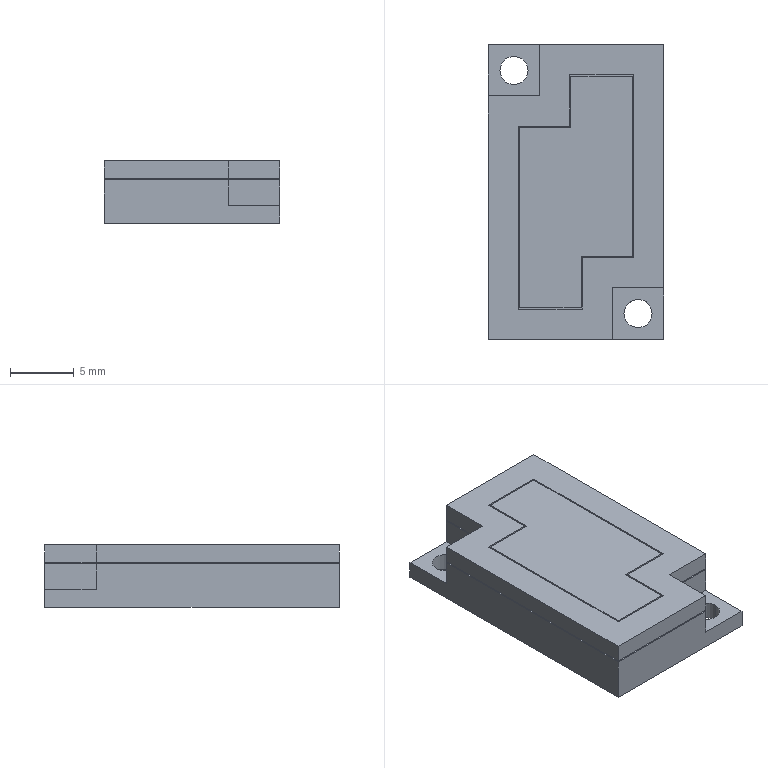Part | SolidWorks | features HoleWzd 2, BaseBody 1, ICE 1 | 1 solid | 52 faces | box 13.7 x 23 x 4.9 mm | volume 1409 mm3 | plane 48 | cylinder 4 | commonest cylinder face diameters 2.2 x4
STEP:
#1=CARTESIAN_POINT('',(8.6,-19.,0.));
#2=VERTEX_POINT('',#1);
#3=CARTESIAN_POINT('',(10.8,-19.,0.));
#4=VERTEX_POINT('',#3);
#5=CARTESIAN_POINT('',(9.7,-19.,0.));
#6=DIRECTION('',(0.,0.,1.));
#7=DIRECTION('',(1.,0.,0.));
#8=AXIS2_PLACEMENT_3D('',#5,#6,#7);
#9=CIRCLE('',#8,1.1);
#10=EDGE_CURVE('',#2,#4,#9,.T.);
#11=ORIENTED_EDGE('',*,*,#10,.F.);
#12=CARTESIAN_POINT('',(8.6,-19.,1.4));
#13=VERTEX_POINT('',#12);
#14=CARTESIAN_POINT('',(8.6,-19.,1.4));
#15=DIRECTION('',(0.,0.,1.));
#16=VECTOR('',#15,1000.);
#17=LINE('',#14,#16);
#18=EDGE_CURVE('',#2,#13,#17,.T.);
#19=ORIENTED_EDGE('',*,*,#18,.T.);
#20=CARTESIAN_POINT('',(10.8,-19.,1.4));
#21=VERTEX_POINT('',#20);
#22=CARTESIAN_POINT('',(9.7,-19.,1.4));
#23=DIRECTION('',(0.,0.,1.));
#24=DIRECTION('',(1.,0.,0.));
#25=AXIS2_PLACEMENT_3D('',#22,#23,#24);
#26=CIRCLE('',#25,1.1);
#27=EDGE_CURVE('',#13,#21,#26,.T.);
#28=ORIENTED_EDGE('',*,*,#27,.T.);
#29=CARTESIAN_POINT('',(10.8,-19.,1.4));
#30=DIRECTION('',(0.,0.,1.));
#31=VECTOR('',#30,1000.);
#32=LINE('',#29,#31);
#33=EDGE_CURVE('',#4,#21,#32,.T.);
#34=ORIENTED_EDGE('',*,*,#33,.F.);
#35=EDGE_LOOP('',(#11,#19,#28,#34));
#36=FACE_OUTER_BOUND('',#35,.T.);
#37=CARTESIAN_POINT('',(9.7,-19.,1.4));
#38=DIRECTION('',(0.,0.,1.));
#39=DIRECTION('',(1.,0.,0.));
#40=AXIS2_PLACEMENT_3D('',#37,#38,#39);
#41=CYLINDRICAL_SURFACE('',#40,1.1);
#42=ADVANCED_FACE('',(#36),#41,.F.);
#43=CARTESIAN_POINT('',(-1.1,0.,0.));
#44=VERTEX_POINT('',#43);
#45=CARTESIAN_POINT('',(1.1,0.,0.));
#46=VERTEX_POINT('',#45);
#47=CARTESIAN_POINT('',(0.,0.,0.));
#48=DIRECTION('',(0.,0.,1.));
#49=DIRECTION('',(1.,0.,0.));
#50=AXIS2_PLACEMENT_3D('',#47,#48,#49);
#51=CIRCLE('',#50,1.1);
#52=EDGE_CURVE('',#44,#46,#51,.T.);
#53=ORIENTED_EDGE('',*,*,#52,.F.);
#54=CARTESIAN_POINT('',(-1.1,0.,1.4));
#55=VERTEX_POINT('',#54);
#56=CARTESIAN_POINT('',(-1.1,0.,1.4));
#57=DIRECTION('',(0.,0.,1.));
#58=VECTOR('',#57,1000.);
#59=LINE('',#56,#58);
#60=EDGE_CURVE('',#44,#55,#59,.T.);
#61=ORIENTED_EDGE('',*,*,#60,.T.);
#62=CARTESIAN_POINT('',(1.1,0.,1.4));
#63=VERTEX_POINT('',#62);
#64=CARTESIAN_POINT('',(0.,0.,1.4));
#65=DIRECTION('',(0.,0.,1.));
#66=DIRECTION('',(1.,0.,0.));
#67=AXIS2_PLACEMENT_3D('',#64,#65,#66);
#68=CIRCLE('',#67,1.1);
#69=EDGE_CURVE('',#55,#63,#68,.T.);
#70=ORIENTED_EDGE('',*,*,#69,.T.);
#71=CARTESIAN_POINT('',(1.1,0.,1.4));
#72=DIRECTION('',(0.,0.,1.));
#73=VECTOR('',#72,1000.);
#74=LINE('',#71,#73);
#75=EDGE_CURVE('',#46,#63,#74,.T.);
#76=ORIENTED_EDGE('',*,*,#75,.F.);
#77=EDGE_LOOP('',(#53,#61,#70,#76));
#78=FACE_OUTER_BOUND('',#77,.T.);
#79=CARTESIAN_POINT('',(0.,0.,1.4));
#80=DIRECTION('',(0.,0.,1.));
#81=DIRECTION('',(1.,0.,0.));
#82=AXIS2_PLACEMENT_3D('',#79,#80,#81);
#83=CYLINDRICAL_SURFACE('',#82,1.1);
#84=ADVANCED_FACE('',(#78),#83,.F.);
#85=CARTESIAN_POINT('',(-2.,-2.,3.5));
#86=VERTEX_POINT('',#85);
#87=CARTESIAN_POINT('',(-2.,-21.,3.5));
#88=VERTEX_POINT('',#87);
#89=CARTESIAN_POINT('',(-2.,-2.,3.5));
#90=DIRECTION('',(0.,-1.,0.));
#91=VECTOR('',#90,1000.);
#92=LINE('',#89,#91);
#93=EDGE_CURVE('',#86,#88,#92,.T.);
#94=ORIENTED_EDGE('',*,*,#93,.T.);
#95=CARTESIAN_POINT('',(-2.,-21.,4.9));
#96=VERTEX_POINT('',#95);
#97=CARTESIAN_POINT('',(-2.,-21.,1.4));
#98=DIRECTION('',(0.,0.,-1.));
#99=VECTOR('',#98,1000.);
#100=LINE('',#97,#99);
#101=EDGE_CURVE('',#96,#88,#100,.T.);
#102=ORIENTED_EDGE('',*,*,#101,.F.);
#103=CARTESIAN_POINT('',(-2.,-2.,4.9));
#104=VERTEX_POINT('',#103);
#105=CARTESIAN_POINT('',(-2.,-2.,4.9));
#106=DIRECTION('',(0.,-1.,0.));
#107=VECTOR('',#106,1000.);
#108=LINE('',#105,#107);
#109=EDGE_CURVE('',#104,#96,#108,.T.);
#110=ORIENTED_EDGE('',*,*,#109,.F.);
#111=CARTESIAN_POINT('',(-2.,-2.,4.9));
#112=DIRECTION('',(0.,0.,-1.));
#113=VECTOR('',#112,1000.);
#114=LINE('',#111,#113);
#115=EDGE_CURVE('',#104,#86,#114,.T.);
#116=ORIENTED_EDGE('',*,*,#115,.T.);
#117=EDGE_LOOP('',(#94,#102,#110,#116));
#118=FACE_OUTER_BOUND('',#117,.T.);
#119=CARTESIAN_POINT('',(-2.,2.,1.4));
#120=DIRECTION('',(1.,0.,0.));
#121=DIRECTION('',(0.,1.,0.));
#122=AXIS2_PLACEMENT_3D('',#119,#120,#121);
#123=PLANE('',#122);
#124=ADVANCED_FACE('',(#118),#123,.F.);
#125=CARTESIAN_POINT('',(7.7,-21.,3.5));
#126=VERTEX_POINT('',#125);
#127=CARTESIAN_POINT('',(-2.,-21.,3.5));
#128=DIRECTION('',(1.,0.,0.));
#129=VECTOR('',#128,1000.);
#130=LINE('',#127,#129);
#131=EDGE_CURVE('',#88,#126,#130,.T.);
#132=ORIENTED_EDGE('',*,*,#131,.T.);
#133=CARTESIAN_POINT('',(7.7,-21.,4.9));
#134=VERTEX_POINT('',#133);
#135=CARTESIAN_POINT('',(7.7,-21.,4.9));
#136=DIRECTION('',(0.,0.,-1.));
#137=VECTOR('',#136,1000.);
#138=LINE('',#135,#137);
#139=EDGE_CURVE('',#134,#126,#138,.T.);
#140=ORIENTED_EDGE('',*,*,#139,.F.);
#141=CARTESIAN_POINT('',(-2.,-21.,4.9));
#142=DIRECTION('',(1.,0.,0.));
#143=VECTOR('',#142,1000.);
#144=LINE('',#141,#143);
#145=EDGE_CURVE('',#96,#134,#144,.T.);
#146=ORIENTED_EDGE('',*,*,#145,.F.);
#147=ORIENTED_EDGE('',*,*,#101,.T.);
#148=EDGE_LOOP('',(#132,#140,#146,#147));
#149=FACE_OUTER_BOUND('',#148,.T.);
#150=CARTESIAN_POINT('',(-2.,-21.,1.4));
#151=DIRECTION('',(0.,1.,0.));
#152=DIRECTION('',(-1.,0.,0.));
#153=AXIS2_PLACEMENT_3D('',#150,#151,#152);
#154=PLANE('',#153);
#155=ADVANCED_FACE('',(#149),#154,.F.);
#156=CARTESIAN_POINT('',(11.7,-17.,3.5));
#157=VERTEX_POINT('',#156);
#158=CARTESIAN_POINT('',(11.7,2.,3.5));
#159=VERTEX_POINT('',#158);
#160=CARTESIAN_POINT('',(11.7,-17.,3.5));
#161=DIRECTION('',(0.,1.,0.));
#162=VECTOR('',#161,1000.);
#163=LINE('',#160,#162);
#164=EDGE_CURVE('',#157,#159,#163,.T.);
#165=ORIENTED_EDGE('',*,*,#164,.T.);
#166=CARTESIAN_POINT('',(11.7,2.,4.9));
#167=VERTEX_POINT('',#166);
#168=CARTESIAN_POINT('',(11.7,2.,1.4));
#169=DIRECTION('',(0.,0.,-1.));
#170=VECTOR('',#169,1000.);
#171=LINE('',#168,#170);
#172=EDGE_CURVE('',#167,#159,#171,.T.);
#173=ORIENTED_EDGE('',*,*,#172,.F.);
#174=CARTESIAN_POINT('',(11.7,-17.,4.9));
#175=VERTEX_POINT('',#174);
#176=CARTESIAN_POINT('',(11.7,-17.,4.9));
#177=DIRECTION('',(0.,1.,0.));
#178=VECTOR('',#177,1000.);
#179=LINE('',#176,#178);
#180=EDGE_CURVE('',#175,#167,#179,.T.);
#181=ORIENTED_EDGE('',*,*,#180,.F.);
#182=CARTESIAN_POINT('',(11.7,-17.,4.9));
#183=DIRECTION('',(0.,0.,-1.));
#184=VECTOR('',#183,1000.);
#185=LINE('',#182,#184);
#186=EDGE_CURVE('',#175,#157,#185,.T.);
#187=ORIENTED_EDGE('',*,*,#186,.T.);
#188=EDGE_LOOP('',(#165,#173,#181,#187));
#189=FACE_OUTER_BOUND('',#188,.T.);
#190=CARTESIAN_POINT('',(11.7,2.,1.4));
#191=DIRECTION('',(-1.,0.,0.));
#192=DIRECTION('',(0.,-1.,0.));
#193=AXIS2_PLACEMENT_3D('',#190,#191,#192);
#194=PLANE('',#193);
#195=ADVANCED_FACE('',(#189),#194,.F.);
#196=CARTESIAN_POINT('',(2.,2.,3.5));
#197=VERTEX_POINT('',#196);
#198=CARTESIAN_POINT('',(11.7,2.,3.5));
#199=DIRECTION('',(-1.,0.,0.));
#200=VECTOR('',#199,1000.);
#201=LINE('',#198,#200);
#202=EDGE_CURVE('',#159,#197,#201,.T.);
#203=ORIENTED_EDGE('',*,*,#202,.T.);
#204=CARTESIAN_POINT('',(2.,2.,4.9));
#205=VERTEX_POINT('',#204);
#206=CARTESIAN_POINT('',(2.,2.,4.9));
#207=DIRECTION('',(0.,0.,-1.));
#208=VECTOR('',#207,1000.);
#209=LINE('',#206,#208);
#210=EDGE_CURVE('',#205,#197,#209,.T.);
#211=ORIENTED_EDGE('',*,*,#210,.F.);
#212=CARTESIAN_POINT('',(11.7,2.,4.9));
#213=DIRECTION('',(-1.,0.,0.));
#214=VECTOR('',#213,1000.);
#215=LINE('',#212,#214);
#216=EDGE_CURVE('',#167,#205,#215,.T.);
#217=ORIENTED_EDGE('',*,*,#216,.F.);
#218=ORIENTED_EDGE('',*,*,#172,.T.);
#219=EDGE_LOOP('',(#203,#211,#217,#218));
#220=FACE_OUTER_BOUND('',#219,.T.);
#221=CARTESIAN_POINT('',(-2.,2.,1.4));
#222=DIRECTION('',(0.,-1.,0.));
#223=DIRECTION('',(1.,0.,0.));
#224=AXIS2_PLACEMENT_3D('',#221,#222,#223);
#225=PLANE('',#224);
#226=ADVANCED_FACE('',(#220),#225,.F.);
#227=CARTESIAN_POINT('',(7.7,-17.,3.5));
#228=VERTEX_POINT('',#227);
#229=CARTESIAN_POINT('',(7.7,-21.,3.5));
#230=DIRECTION('',(0.,1.,0.));
#231=VECTOR('',#230,1000.);
#232=LINE('',#229,#231);
#233=EDGE_CURVE('',#126,#228,#232,.T.);
#234=ORIENTED_EDGE('',*,*,#233,.T.);
#235=CARTESIAN_POINT('',(7.7,-17.,4.9));
#236=VERTEX_POINT('',#235);
#237=CARTESIAN_POINT('',(7.7,-17.,4.9));
#238=DIRECTION('',(0.,0.,-1.));
#239=VECTOR('',#238,1000.);
#240=LINE('',#237,#239);
#241=EDGE_CURVE('',#236,#228,#240,.T.);
#242=ORIENTED_EDGE('',*,*,#241,.F.);
#243=CARTESIAN_POINT('',(7.7,-17.,4.9));
#244=DIRECTION('',(0.,1.,0.));
#245=VECTOR('',#244,1000.);
#246=LINE('',#243,#245);
#247=EDGE_CURVE('',#134,#236,#246,.T.);
#248=ORIENTED_EDGE('',*,*,#247,.F.);
#249=ORIENTED_EDGE('',*,*,#139,.T.);
#250=EDGE_LOOP('',(#234,#242,#248,#249));
#251=FACE_OUTER_BOUND('',#250,.T.);
#252=CARTESIAN_POINT('',(7.7,-17.,4.9));
#253=DIRECTION('',(-1.,0.,0.));
#254=DIRECTION('',(0.,0.,1.));
#255=AXIS2_PLACEMENT_3D('',#252,#253,#254);
#256=PLANE('',#255);
#257=ADVANCED_FACE('',(#251),#256,.F.);
#258=CARTESIAN_POINT('',(7.7,-17.,3.5));
#259=DIRECTION('',(1.,0.,0.));
#260=VECTOR('',#259,1000.);
#261=LINE('',#258,#260);
#262=EDGE_CURVE('',#228,#157,#261,.T.);
#263=ORIENTED_EDGE('',*,*,#262,.T.);
#264=ORIENTED_EDGE('',*,*,#186,.F.);
#265=CARTESIAN_POINT('',(7.7,-17.,4.9));
#266=DIRECTION('',(1.,0.,0.));
#267=VECTOR('',#266,1000.);
#268=LINE('',#265,#267);
#269=EDGE_CURVE('',#236,#175,#268,.T.);
#270=ORIENTED_EDGE('',*,*,#269,.F.);
#271=ORIENTED_EDGE('',*,*,#241,.T.);
#272=EDGE_LOOP('',(#263,#264,#270,#271));
#273=FACE_OUTER_BOUND('',#272,.T.);
#274=CARTESIAN_POINT('',(7.7,-17.,4.9));
#275=DIRECTION('',(0.,1.,0.));
#276=DIRECTION('',(0.,0.,1.));
#277=AXIS2_PLACEMENT_3D('',#274,#275,#276);
#278=PLANE('',#277);
#279=ADVANCED_FACE('',(#273),#278,.F.);
#280=CARTESIAN_POINT('',(2.,-2.,3.5));
#281=VERTEX_POINT('',#280);
#282=CARTESIAN_POINT('',(2.,2.,3.5));
#283=DIRECTION('',(0.,-1.,0.));
#284=VECTOR('',#283,1000.);
#285=LINE('',#282,#284);
#286=EDGE_CURVE('',#197,#281,#285,.T.);
#287=ORIENTED_EDGE('',*,*,#286,.T.);
#288=CARTESIAN_POINT('',(2.,-2.,4.9));
#289=VERTEX_POINT('',#288);
#290=CARTESIAN_POINT('',(2.,-2.,4.9));
#291=DIRECTION('',(0.,0.,-1.));
#292=VECTOR('',#291,1000.);
#293=LINE('',#290,#292);
#294=EDGE_CURVE('',#289,#281,#293,.T.);
#295=ORIENTED_EDGE('',*,*,#294,.F.);
#296=CARTESIAN_POINT('',(2.,2.,4.9));
#297=DIRECTION('',(0.,-1.,0.));
#298=VECTOR('',#297,1000.);
#299=LINE('',#296,#298);
#300=EDGE_CURVE('',#205,#289,#299,.T.);
#301=ORIENTED_EDGE('',*,*,#300,.F.);
#302=ORIENTED_EDGE('',*,*,#210,.T.);
#303=EDGE_LOOP('',(#287,#295,#301,#302));
#304=FACE_OUTER_BOUND('',#303,.T.);
#305=CARTESIAN_POINT('',(2.,2.,4.9));
#306=DIRECTION('',(1.,0.,0.));
#307=DIRECTION('',(0.,1.,0.));
#308=AXIS2_PLACEMENT_3D('',#305,#306,#307);
#309=PLANE('',#308);
#310=ADVANCED_FACE('',(#304),#309,.F.);
#311=CARTESIAN_POINT('',(2.,-2.,3.5));
#312=DIRECTION('',(-1.,0.,0.));
#313=VECTOR('',#312,1000.);
#314=LINE('',#311,#313);
#315=EDGE_CURVE('',#281,#86,#314,.T.);
#316=ORIENTED_EDGE('',*,*,#315,.T.);
#317=ORIENTED_EDGE('',*,*,#115,.F.);
#318=CARTESIAN_POINT('',(2.,-2.,4.9));
#319=DIRECTION('',(-1.,0.,0.));
#320=VECTOR('',#319,1000.);
#321=LINE('',#318,#320);
#322=EDGE_CURVE('',#289,#104,#321,.T.);
#323=ORIENTED_EDGE('',*,*,#322,.F.);
#324=ORIENTED_EDGE('',*,*,#294,.T.);
#325=EDGE_LOOP('',(#316,#317,#323,#324));
#326=FACE_OUTER_BOUND('',#325,.T.);
#327=CARTESIAN_POINT('',(2.,-2.,4.9));
#328=DIRECTION('',(0.,-1.,0.));
#329=DIRECTION('',(1.,0.,0.));
#330=AXIS2_PLACEMENT_3D('',#327,#328,#329);
#331=PLANE('',#330);
#332=ADVANCED_FACE('',(#326),#331,.F.);
#333=CARTESIAN_POINT('',(0.35,-4.35,4.9));
#334=VERTEX_POINT('',#333);
#335=CARTESIAN_POINT('',(0.35,-18.65,4.9));
#336=VERTEX_POINT('',#335);
#337=CARTESIAN_POINT('',(0.35,-4.45,4.9));
#338=DIRECTION('',(0.,-1.,0.));
#339=VECTOR('',#338,1000.);
#340=LINE('',#337,#339);
#341=EDGE_CURVE('',#334,#336,#340,.T.);
#342=ORIENTED_EDGE('',*,*,#341,.F.);
#343=CARTESIAN_POINT('',(4.35,-4.35,4.9));
#344=VERTEX_POINT('',#343);
#345=CARTESIAN_POINT('',(0.45,-4.35,4.9));
#346=DIRECTION('',(-1.,0.,0.));
#347=VECTOR('',#346,1000.);
#348=LINE('',#345,#347);
#349=EDGE_CURVE('',#344,#334,#348,.T.);
#350=ORIENTED_EDGE('',*,*,#349,.F.);
#351=CARTESIAN_POINT('',(4.35,-0.35,4.9));
#352=VERTEX_POINT('',#351);
#353=CARTESIAN_POINT('',(4.35,-4.45,4.9));
#354=DIRECTION('',(0.,-1.,0.));
#355=VECTOR('',#354,1000.);
#356=LINE('',#353,#355);
#357=EDGE_CURVE('',#352,#344,#356,.T.);
#358=ORIENTED_EDGE('',*,*,#357,.F.);
#359=CARTESIAN_POINT('',(9.35,-0.35,4.9));
#360=VERTEX_POINT('',#359);
#361=CARTESIAN_POINT('',(0.45,-0.35,4.9));
#362=DIRECTION('',(-1.,0.,0.));
#363=VECTOR('',#362,1000.);
#364=LINE('',#361,#363);
#365=EDGE_CURVE('',#360,#352,#364,.T.);
#366=ORIENTED_EDGE('',*,*,#365,.F.);
#367=CARTESIAN_POINT('',(9.35,-14.65,4.9));
#368=VERTEX_POINT('',#367);
#369=CARTESIAN_POINT('',(9.35,-4.45,4.9));
#370=DIRECTION('',(0.,1.,0.));
#371=VECTOR('',#370,1000.);
#372=LINE('',#369,#371);
#373=EDGE_CURVE('',#368,#360,#372,.T.);
#374=ORIENTED_EDGE('',*,*,#373,.F.);
#375=CARTESIAN_POINT('',(5.35,-14.65,4.9));
#376=VERTEX_POINT('',#375);
#377=CARTESIAN_POINT('',(0.45,-14.65,4.9));
#378=DIRECTION('',(1.,0.,0.));
#379=VECTOR('',#378,1000.);
#380=LINE('',#377,#379);
#381=EDGE_CURVE('',#376,#368,#380,.T.);
#382=ORIENTED_EDGE('',*,*,#381,.F.);
#383=CARTESIAN_POINT('',(5.35,-18.65,4.9));
#384=VERTEX_POINT('',#383);
#385=CARTESIAN_POINT('',(5.35,-4.45,4.9));
#386=DIRECTION('',(0.,1.,0.));
#387=VECTOR('',#386,1000.);
#388=LINE('',#385,#387);
#389=EDGE_CURVE('',#384,#376,#388,.T.);
#390=ORIENTED_EDGE('',*,*,#389,.F.);
#391=CARTESIAN_POINT('',(0.45,-18.65,4.9));
#392=DIRECTION('',(1.,0.,0.));
#393=VECTOR('',#392,1000.);
#394=LINE('',#391,#393);
#395=EDGE_CURVE('',#336,#384,#394,.T.);
#396=ORIENTED_EDGE('',*,*,#395,.F.);
#397=EDGE_LOOP('',(#342,#350,#358,#366,#374,#382,#390,#396));
#398=FACE_BOUND('',#397,.T.);
#399=ORIENTED_EDGE('',*,*,#145,.T.);
#400=ORIENTED_EDGE('',*,*,#247,.T.);
#401=ORIENTED_EDGE('',*,*,#269,.T.);
#402=ORIENTED_EDGE('',*,*,#180,.T.);
#403=ORIENTED_EDGE('',*,*,#216,.T.);
#404=ORIENTED_EDGE('',*,*,#300,.T.);
#405=ORIENTED_EDGE('',*,*,#322,.T.);
#406=ORIENTED_EDGE('',*,*,#109,.T.);
#407=EDGE_LOOP('',(#399,#400,#401,#402,#403,#404,#405,#406));
#408=FACE_OUTER_BOUND('',#407,.T.);
#409=CARTESIAN_POINT('',(11.7,-21.,4.9));
#410=DIRECTION('',(0.,0.,1.));
#411=DIRECTION('',(1.,0.,0.));
#412=AXIS2_PLACEMENT_3D('',#409,#410,#411);
#413=PLANE('',#412);
#414=ADVANCED_FACE('',(#398,#408),#413,.T.);
#415=ORIENTED_EDGE('',*,*,#341,.T.);
#416=CARTESIAN_POINT('',(0.35,-18.65,3.9));
#417=VERTEX_POINT('',#416);
#418=CARTESIAN_POINT('',(0.35,-18.65,3.9));
#419=DIRECTION('',(0.,0.,1.));
#420=VECTOR('',#419,1000.);
#421=LINE('',#418,#420);
#422=EDGE_CURVE('',#417,#336,#421,.T.);
#423=ORIENTED_EDGE('',*,*,#422,.F.);
#424=CARTESIAN_POINT('',(0.35,-4.35,3.9));
#425=VERTEX_POINT('',#424);
#426=CARTESIAN_POINT('',(0.35,-4.45,3.9));
#427=DIRECTION('',(0.,-1.,0.));
#428=VECTOR('',#427,1000.);
#429=LINE('',#426,#428);
#430=EDGE_CURVE('',#425,#417,#429,.T.);
#431=ORIENTED_EDGE('',*,*,#430,.F.);
#432=CARTESIAN_POINT('',(0.35,-4.35,3.9));
#433=DIRECTION('',(0.,0.,1.));
#434=VECTOR('',#433,1000.);
#435=LINE('',#432,#434);
#436=EDGE_CURVE('',#425,#334,#435,.T.);
#437=ORIENTED_EDGE('',*,*,#436,.T.);
#438=EDGE_LOOP('',(#415,#423,#431,#437));
#439=FACE_OUTER_BOUND('',#438,.T.);
#440=CARTESIAN_POINT('',(0.35,-4.45,3.9));
#441=DIRECTION('',(-1.,0.,0.));
#442=DIRECTION('',(0.,-1.,0.));
#443=AXIS2_PLACEMENT_3D('',#440,#441,#442);
#444=PLANE('',#443);
#445=ADVANCED_FACE('',(#439),#444,.F.);
#446=ORIENTED_EDGE('',*,*,#349,.T.);
#447=ORIENTED_EDGE('',*,*,#436,.F.);
#448=CARTESIAN_POINT('',(4.35,-4.35,3.9));
#449=VERTEX_POINT('',#448);
#450=CARTESIAN_POINT('',(0.45,-4.35,3.9));
#451=DIRECTION('',(-1.,0.,0.));
#452=VECTOR('',#451,1000.);
#453=LINE('',#450,#452);
#454=EDGE_CURVE('',#449,#425,#453,.T.);
#455=ORIENTED_EDGE('',*,*,#454,.F.);
#456=CARTESIAN_POINT('',(4.35,-4.35,3.9));
#457=DIRECTION('',(0.,0.,1.));
#458=VECTOR('',#457,1000.);
#459=LINE('',#456,#458);
#460=EDGE_CURVE('',#449,#344,#459,.T.);
#461=ORIENTED_EDGE('',*,*,#460,.T.);
#462=EDGE_LOOP('',(#446,#447,#455,#461));
#463=FACE_OUTER_BOUND('',#462,.T.);
#464=CARTESIAN_POINT('',(0.45,-4.35,3.9));
#465=DIRECTION('',(0.,1.,0.));
#466=DIRECTION('',(-1.,0.,0.));
#467=AXIS2_PLACEMENT_3D('',#464,#465,#466);
#468=PLANE('',#467);
#469=ADVANCED_FACE('',(#463),#468,.F.);
#470=ORIENTED_EDGE('',*,*,#357,.T.);
#471=ORIENTED_EDGE('',*,*,#460,.F.);
#472=CARTESIAN_POINT('',(4.35,-0.35,3.9));
#473=VERTEX_POINT('',#472);
#474=CARTESIAN_POINT('',(4.35,-4.45,3.9));
#475=DIRECTION('',(0.,-1.,0.));
#476=VECTOR('',#475,1000.);
#477=LINE('',#474,#476);
#478=EDGE_CURVE('',#473,#449,#477,.T.);
#479=ORIENTED_EDGE('',*,*,#478,.F.);
#480=CARTESIAN_POINT('',(4.35,-0.35,3.9));
#481=DIRECTION('',(0.,0.,1.));
#482=VECTOR('',#481,1000.);
#483=LINE('',#480,#482);
#484=EDGE_CURVE('',#473,#352,#483,.T.);
#485=ORIENTED_EDGE('',*,*,#484,.T.);
#486=EDGE_LOOP('',(#470,#471,#479,#485));
#487=FACE_OUTER_BOUND('',#486,.T.);
#488=CARTESIAN_POINT('',(4.35,-4.45,3.9));
#489=DIRECTION('',(-1.,0.,0.));
#490=DIRECTION('',(0.,-1.,0.));
#491=AXIS2_PLACEMENT_3D('',#488,#489,#490);
#492=PLANE('',#491);
#493=ADVANCED_FACE('',(#487),#492,.F.);
#494=ORIENTED_EDGE('',*,*,#365,.T.);
#495=ORIENTED_EDGE('',*,*,#484,.F.);
#496=CARTESIAN_POINT('',(9.35,-0.35,3.9));
#497=VERTEX_POINT('',#496);
#498=CARTESIAN_POINT('',(0.45,-0.35,3.9));
#499=DIRECTION('',(-1.,0.,0.));
#500=VECTOR('',#499,1000.);
#501=LINE('',#498,#500);
#502=EDGE_CURVE('',#497,#473,#501,.T.);
#503=ORIENTED_EDGE('',*,*,#502,.F.);
#504=CARTESIAN_POINT('',(9.35,-0.35,3.9));
#505=DIRECTION('',(0.,0.,1.));
#506=VECTOR('',#505,1000.);
#507=LINE('',#504,#506);
#508=EDGE_CURVE('',#497,#360,#507,.T.);
#509=ORIENTED_EDGE('',*,*,#508,.T.);
#510=EDGE_LOOP('',(#494,#495,#503,#509));
#511=FACE_OUTER_BOUND('',#510,.T.);
#512=CARTESIAN_POINT('',(0.45,-0.35,3.9));
#513=DIRECTION('',(0.,1.,0.));
#514=DIRECTION('',(-1.,0.,0.));
#515=AXIS2_PLACEMENT_3D('',#512,#513,#514);
#516=PLANE('',#515);
#517=ADVANCED_FACE('',(#511),#516,.F.);
#518=ORIENTED_EDGE('',*,*,#373,.T.);
#519=ORIENTED_EDGE('',*,*,#508,.F.);
#520=CARTESIAN_POINT('',(9.35,-14.65,3.9));
#521=VERTEX_POINT('',#520);
#522=CARTESIAN_POINT('',(9.35,-4.45,3.9));
#523=DIRECTION('',(0.,1.,0.));
#524=VECTOR('',#523,1000.);
#525=LINE('',#522,#524);
#526=EDGE_CURVE('',#521,#497,#525,.T.);
#527=ORIENTED_EDGE('',*,*,#526,.F.);
#528=CARTESIAN_POINT('',(9.35,-14.65,3.9));
#529=DIRECTION('',(0.,0.,1.));
#530=VECTOR('',#529,1000.);
#531=LINE('',#528,#530);
#532=EDGE_CURVE('',#521,#368,#531,.T.);
#533=ORIENTED_EDGE('',*,*,#532,.T.);
#534=EDGE_LOOP('',(#518,#519,#527,#533));
#535=FACE_OUTER_BOUND('',#534,.T.);
#536=CARTESIAN_POINT('',(9.35,-4.45,3.9));
#537=DIRECTION('',(1.,0.,0.));
#538=DIRECTION('',(0.,1.,0.));
#539=AXIS2_PLACEMENT_3D('',#536,#537,#538);
#540=PLANE('',#539);
#541=ADVANCED_FACE('',(#535),#540,.F.);
#542=ORIENTED_EDGE('',*,*,#381,.T.);
#543=ORIENTED_EDGE('',*,*,#532,.F.);
#544=CARTESIAN_POINT('',(5.35,-14.65,3.9));
#545=VERTEX_POINT('',#544);
#546=CARTESIAN_POINT('',(0.45,-14.65,3.9));
#547=DIRECTION('',(1.,0.,0.));
#548=VECTOR('',#547,1000.);
#549=LINE('',#546,#548);
#550=EDGE_CURVE('',#545,#521,#549,.T.);
#551=ORIENTED_EDGE('',*,*,#550,.F.);
#552=CARTESIAN_POINT('',(5.35,-14.65,3.9));
#553=DIRECTION('',(0.,0.,1.));
#554=VECTOR('',#553,1000.);
#555=LINE('',#552,#554);
#556=EDGE_CURVE('',#545,#376,#555,.T.);
#557=ORIENTED_EDGE('',*,*,#556,.T.);
#558=EDGE_LOOP('',(#542,#543,#551,#557));
#559=FACE_OUTER_BOUND('',#558,.T.);
#560=CARTESIAN_POINT('',(0.45,-14.65,3.9));
#561=DIRECTION('',(0.,-1.,0.));
#562=DIRECTION('',(0.,0.,-1.));
#563=AXIS2_PLACEMENT_3D('',#560,#561,#562);
#564=PLANE('',#563);
#565=ADVANCED_FACE('',(#559),#564,.F.);
#566=ORIENTED_EDGE('',*,*,#389,.T.);
#567=ORIENTED_EDGE('',*,*,#556,.F.);
#568=CARTESIAN_POINT('',(5.35,-18.65,3.9));
#569=VERTEX_POINT('',#568);
#570=CARTESIAN_POINT('',(5.35,-4.45,3.9));
#571=DIRECTION('',(0.,1.,0.));
#572=VECTOR('',#571,1000.);
#573=LINE('',#570,#572);
#574=EDGE_CURVE('',#569,#545,#573,.T.);
#575=ORIENTED_EDGE('',*,*,#574,.F.);
#576=CARTESIAN_POINT('',(5.35,-18.65,3.9));
#577=DIRECTION('',(0.,0.,1.));
#578=VECTOR('',#577,1000.);
#579=LINE('',#576,#578);
#580=EDGE_CURVE('',#569,#384,#579,.T.);
#581=ORIENTED_EDGE('',*,*,#580,.T.);
#582=EDGE_LOOP('',(#566,#567,#575,#581));
#583=FACE_OUTER_BOUND('',#582,.T.);
#584=CARTESIAN_POINT('',(5.35,-4.45,3.9));
#585=DIRECTION('',(1.,0.,0.));
#586=DIRECTION('',(0.,0.,-1.));
#587=AXIS2_PLACEMENT_3D('',#584,#585,#586);
#588=PLANE('',#587);
#589=ADVANCED_FACE('',(#583),#588,.F.);
#590=ORIENTED_EDGE('',*,*,#395,.T.);
#591=ORIENTED_EDGE('',*,*,#580,.F.);
#592=CARTESIAN_POINT('',(0.45,-18.65,3.9));
#593=DIRECTION('',(1.,0.,0.));
#594=VECTOR('',#593,1000.);
#595=LINE('',#592,#594);
#596=EDGE_CURVE('',#417,#569,#595,.T.);
#597=ORIENTED_EDGE('',*,*,#596,.F.);
#598=ORIENTED_EDGE('',*,*,#422,.T.);
#599=EDGE_LOOP('',(#590,#591,#597,#598));
#600=FACE_OUTER_BOUND('',#599,.T.);
#601=CARTESIAN_POINT('',(0.45,-18.65,3.9));
#602=DIRECTION('',(0.,-1.,0.));
#603=DIRECTION('',(0.,0.,-1.));
#604=AXIS2_PLACEMENT_3D('',#601,#602,#603);
#605=PLANE('',#604);
#606=ADVANCED_FACE('',(#600),#605,.F.);
#607=CARTESIAN_POINT('',(0.45,-4.45,3.9));
#608=VERTEX_POINT('',#607);
#609=CARTESIAN_POINT('',(0.45,-18.55,3.9));
#610=VERTEX_POINT('',#609);
#611=CARTESIAN_POINT('',(0.45,-4.45,3.9));
#612=DIRECTION('',(0.,-1.,0.));
#613=VECTOR('',#612,1000.);
#614=LINE('',#611,#613);
#615=EDGE_CURVE('',#608,#610,#614,.T.);
#616=ORIENTED_EDGE('',*,*,#615,.F.);
#617=CARTESIAN_POINT('',(4.45,-4.45,3.9));
#618=VERTEX_POINT('',#617);
#619=CARTESIAN_POINT('',(4.45,-4.45,3.9));
#620=DIRECTION('',(-1.,0.,0.));
#621=VECTOR('',#620,1000.);
#622=LINE('',#619,#621);
#623=EDGE_CURVE('',#618,#608,#622,.T.);
#624=ORIENTED_EDGE('',*,*,#623,.F.);
#625=CARTESIAN_POINT('',(4.45,-0.45,3.9));
#626=VERTEX_POINT('',#625);
#627=CARTESIAN_POINT('',(4.45,-0.45,3.9));
#628=DIRECTION('',(0.,-1.,0.));
#629=VECTOR('',#628,1000.);
#630=LINE('',#627,#629);
#631=EDGE_CURVE('',#626,#618,#630,.T.);
#632=ORIENTED_EDGE('',*,*,#631,.F.);
#633=CARTESIAN_POINT('',(9.25,-0.45,3.9));
#634=VERTEX_POINT('',#633);
#635=CARTESIAN_POINT('',(9.25,-0.45,3.9));
#636=DIRECTION('',(-1.,0.,0.));
#637=VECTOR('',#636,1000.);
#638=LINE('',#635,#637);
#639=EDGE_CURVE('',#634,#626,#638,.T.);
#640=ORIENTED_EDGE('',*,*,#639,.F.);
#641=CARTESIAN_POINT('',(9.25,-14.55,3.9));
#642=VERTEX_POINT('',#641);
#643=CARTESIAN_POINT('',(9.25,-14.55,3.9));
#644=DIRECTION('',(0.,1.,0.));
#645=VECTOR('',#644,1000.);
#646=LINE('',#643,#645);
#647=EDGE_CURVE('',#642,#634,#646,.T.);
#648=ORIENTED_EDGE('',*,*,#647,.F.);
#649=CARTESIAN_POINT('',(5.25,-14.55,3.9));
#650=VERTEX_POINT('',#649);
#651=CARTESIAN_POINT('',(5.25,-14.55,3.9));
#652=DIRECTION('',(1.,0.,0.));
#653=VECTOR('',#652,1000.);
#654=LINE('',#651,#653);
#655=EDGE_CURVE('',#650,#642,#654,.T.);
#656=ORIENTED_EDGE('',*,*,#655,.F.);
#657=CARTESIAN_POINT('',(5.25,-18.55,3.9));
#658=VERTEX_POINT('',#657);
#659=CARTESIAN_POINT('',(5.25,-18.55,3.9));
#660=DIRECTION('',(0.,1.,0.));
#661=VECTOR('',#660,1000.);
#662=LINE('',#659,#661);
#663=EDGE_CURVE('',#658,#650,#662,.T.);
#664=ORIENTED_EDGE('',*,*,#663,.F.);
#665=CARTESIAN_POINT('',(0.45,-18.55,3.9));
#666=DIRECTION('',(1.,0.,0.));
#667=VECTOR('',#666,1000.);
#668=LINE('',#665,#667);
#669=EDGE_CURVE('',#610,#658,#668,.T.);
#670=ORIENTED_EDGE('',*,*,#669,.F.);
#671=EDGE_LOOP('',(#616,#624,#632,#640,#648,#656,#664,#670));
#672=FACE_BOUND('',#671,.T.);
#673=ORIENTED_EDGE('',*,*,#430,.T.);
#674=ORIENTED_EDGE('',*,*,#596,.T.);
#675=ORIENTED_EDGE('',*,*,#574,.T.);
#676=ORIENTED_EDGE('',*,*,#550,.T.);
#677=ORIENTED_EDGE('',*,*,#526,.T.);
#678=ORIENTED_EDGE('',*,*,#502,.T.);
#679=ORIENTED_EDGE('',*,*,#478,.T.);
#680=ORIENTED_EDGE('',*,*,#454,.T.);
#681=EDGE_LOOP('',(#673,#674,#675,#676,#677,#678,#679,#680));
#682=FACE_OUTER_BOUND('',#681,.T.);
#683=CARTESIAN_POINT('',(0.35,-4.35,3.9));
#684=DIRECTION('',(0.,0.,-1.));
#685=DIRECTION('',(-1.,0.,0.));
#686=AXIS2_PLACEMENT_3D('',#683,#684,#685);
#687=PLANE('',#686);
#688=ADVANCED_FACE('',(#672,#682),#687,.F.);
#689=CARTESIAN_POINT('',(0.45,-4.45,4.9));
#690=VERTEX_POINT('',#689);
#691=CARTESIAN_POINT('',(0.45,-18.55,4.9));
#692=VERTEX_POINT('',#691);
#693=CARTESIAN_POINT('',(0.45,-4.45,4.9));
#694=DIRECTION('',(0.,-1.,0.));
#695=VECTOR('',#694,1000.);
#696=LINE('',#693,#695);
#697=EDGE_CURVE('',#690,#692,#696,.T.);
#698=ORIENTED_EDGE('',*,*,#697,.F.);
#699=CARTESIAN_POINT('',(0.45,-4.45,3.9));
#700=DIRECTION('',(0.,0.,1.));
#701=VECTOR('',#700,1000.);
#702=LINE('',#699,#701);
#703=EDGE_CURVE('',#608,#690,#702,.T.);
#704=ORIENTED_EDGE('',*,*,#703,.F.);
#705=ORIENTED_EDGE('',*,*,#615,.T.);
#706=CARTESIAN_POINT('',(0.45,-18.55,3.9));
#707=DIRECTION('',(0.,0.,1.));
#708=VECTOR('',#707,1000.);
#709=LINE('',#706,#708);
#710=EDGE_CURVE('',#610,#692,#709,.T.);
#711=ORIENTED_EDGE('',*,*,#710,.T.);
#712=EDGE_LOOP('',(#698,#704,#705,#711));
#713=FACE_OUTER_BOUND('',#712,.T.);
#714=CARTESIAN_POINT('',(0.45,-4.45,3.9));
#715=DIRECTION('',(-1.,0.,0.));
#716=DIRECTION('',(0.,-1.,0.));
#717=AXIS2_PLACEMENT_3D('',#714,#715,#716);
#718=PLANE('',#717);
#719=ADVANCED_FACE('',(#713),#718,.T.);
#720=CARTESIAN_POINT('',(4.45,-4.45,4.9));
#721=VERTEX_POINT('',#720);
#722=CARTESIAN_POINT('',(4.45,-4.45,4.9));
#723=DIRECTION('',(-1.,0.,0.));
#724=VECTOR('',#723,1000.);
#725=LINE('',#722,#724);
#726=EDGE_CURVE('',#721,#690,#725,.T.);
#727=ORIENTED_EDGE('',*,*,#726,.F.);
#728=CARTESIAN_POINT('',(4.45,-4.45,3.9));
#729=DIRECTION('',(0.,0.,1.));
#730=VECTOR('',#729,1000.);
#731=LINE('',#728,#730);
#732=EDGE_CURVE('',#618,#721,#731,.T.);
#733=ORIENTED_EDGE('',*,*,#732,.F.);
#734=ORIENTED_EDGE('',*,*,#623,.T.);
#735=ORIENTED_EDGE('',*,*,#703,.T.);
#736=EDGE_LOOP('',(#727,#733,#734,#735));
#737=FACE_OUTER_BOUND('',#736,.T.);
#738=CARTESIAN_POINT('',(4.45,-4.45,3.9));
#739=DIRECTION('',(0.,1.,0.));
#740=DIRECTION('',(-1.,0.,0.));
#741=AXIS2_PLACEMENT_3D('',#738,#739,#740);
#742=PLANE('',#741);
#743=ADVANCED_FACE('',(#737),#742,.T.);
#744=CARTESIAN_POINT('',(4.45,-0.45,4.9));
#745=VERTEX_POINT('',#744);
#746=CARTESIAN_POINT('',(4.45,-0.45,4.9));
#747=DIRECTION('',(0.,-1.,0.));
#748=VECTOR('',#747,1000.);
#749=LINE('',#746,#748);
#750=EDGE_CURVE('',#745,#721,#749,.T.);
#751=ORIENTED_EDGE('',*,*,#750,.F.);
#752=CARTESIAN_POINT('',(4.45,-0.45,3.9));
#753=DIRECTION('',(0.,0.,1.));
#754=VECTOR('',#753,1000.);
#755=LINE('',#752,#754);
#756=EDGE_CURVE('',#626,#745,#755,.T.);
#757=ORIENTED_EDGE('',*,*,#756,.F.);
#758=ORIENTED_EDGE('',*,*,#631,.T.);
#759=ORIENTED_EDGE('',*,*,#732,.T.);
#760=EDGE_LOOP('',(#751,#757,#758,#759));
#761=FACE_OUTER_BOUND('',#760,.T.);
#762=CARTESIAN_POINT('',(4.45,-0.45,3.9));
#763=DIRECTION('',(-1.,0.,0.));
#764=DIRECTION('',(0.,-1.,0.));
#765=AXIS2_PLACEMENT_3D('',#762,#763,#764);
#766=PLANE('',#765);
#767=ADVANCED_FACE('',(#761),#766,.T.);
#768=CARTESIAN_POINT('',(9.25,-0.45,4.9));
#769=VERTEX_POINT('',#768);
#770=CARTESIAN_POINT('',(9.25,-0.45,4.9));
#771=DIRECTION('',(-1.,0.,0.));
#772=VECTOR('',#771,1000.);
#773=LINE('',#770,#772);
#774=EDGE_CURVE('',#769,#745,#773,.T.);
#775=ORIENTED_EDGE('',*,*,#774,.F.);
#776=CARTESIAN_POINT('',(9.25,-0.45,3.9));
#777=DIRECTION('',(0.,0.,1.));
#778=VECTOR('',#777,1000.);
#779=LINE('',#776,#778);
#780=EDGE_CURVE('',#634,#769,#779,.T.);
#781=ORIENTED_EDGE('',*,*,#780,.F.);
#782=ORIENTED_EDGE('',*,*,#639,.T.);
#783=ORIENTED_EDGE('',*,*,#756,.T.);
#784=EDGE_LOOP('',(#775,#781,#782,#783));
#785=FACE_OUTER_BOUND('',#784,.T.);
#786=CARTESIAN_POINT('',(9.25,-0.45,3.9));
#787=DIRECTION('',(0.,1.,0.));
#788=DIRECTION('',(-1.,0.,0.));
#789=AXIS2_PLACEMENT_3D('',#786,#787,#788);
#790=PLANE('',#789);
#791=ADVANCED_FACE('',(#785),#790,.T.);
#792=CARTESIAN_POINT('',(9.25,-14.55,4.9));
#793=VERTEX_POINT('',#792);
#794=CARTESIAN_POINT('',(9.25,-14.55,4.9));
#795=DIRECTION('',(0.,1.,0.));
#796=VECTOR('',#795,1000.);
#797=LINE('',#794,#796);
#798=EDGE_CURVE('',#793,#769,#797,.T.);
#799=ORIENTED_EDGE('',*,*,#798,.F.);
#800=CARTESIAN_POINT('',(9.25,-14.55,3.9));
#801=DIRECTION('',(0.,0.,1.));
#802=VECTOR('',#801,1000.);
#803=LINE('',#800,#802);
#804=EDGE_CURVE('',#642,#793,#803,.T.);
#805=ORIENTED_EDGE('',*,*,#804,.F.);
#806=ORIENTED_EDGE('',*,*,#647,.T.);
#807=ORIENTED_EDGE('',*,*,#780,.T.);
#808=EDGE_LOOP('',(#799,#805,#806,#807));
#809=FACE_OUTER_BOUND('',#808,.T.);
#810=CARTESIAN_POINT('',(9.25,-14.55,3.9));
#811=DIRECTION('',(1.,0.,0.));
#812=DIRECTION('',(0.,1.,0.));
#813=AXIS2_PLACEMENT_3D('',#810,#811,#812);
#814=PLANE('',#813);
#815=ADVANCED_FACE('',(#809),#814,.T.);
#816=CARTESIAN_POINT('',(5.25,-14.55,4.9));
#817=VERTEX_POINT('',#816);
#818=CARTESIAN_POINT('',(5.25,-14.55,4.9));
#819=DIRECTION('',(1.,0.,0.));
#820=VECTOR('',#819,1000.);
#821=LINE('',#818,#820);
#822=EDGE_CURVE('',#817,#793,#821,.T.);
#823=ORIENTED_EDGE('',*,*,#822,.F.);
#824=CARTESIAN_POINT('',(5.25,-14.55,3.9));
#825=DIRECTION('',(0.,0.,1.));
#826=VECTOR('',#825,1000.);
#827=LINE('',#824,#826);
#828=EDGE_CURVE('',#650,#817,#827,.T.);
#829=ORIENTED_EDGE('',*,*,#828,.F.);
#830=ORIENTED_EDGE('',*,*,#655,.T.);
#831=ORIENTED_EDGE('',*,*,#804,.T.);
#832=EDGE_LOOP('',(#823,#829,#830,#831));
#833=FACE_OUTER_BOUND('',#832,.T.);
#834=CARTESIAN_POINT('',(5.25,-14.55,3.9));
#835=DIRECTION('',(0.,-1.,0.));
#836=DIRECTION('',(0.,0.,-1.));
#837=AXIS2_PLACEMENT_3D('',#834,#835,#836);
#838=PLANE('',#837);
#839=ADVANCED_FACE('',(#833),#838,.T.);
#840=CARTESIAN_POINT('',(5.25,-18.55,4.9));
#841=VERTEX_POINT('',#840);
#842=CARTESIAN_POINT('',(5.25,-18.55,4.9));
#843=DIRECTION('',(0.,1.,0.));
#844=VECTOR('',#843,1000.);
#845=LINE('',#842,#844);
#846=EDGE_CURVE('',#841,#817,#845,.T.);
#847=ORIENTED_EDGE('',*,*,#846,.F.);
#848=CARTESIAN_POINT('',(5.25,-18.55,3.9));
#849=DIRECTION('',(0.,0.,1.));
#850=VECTOR('',#849,1000.);
#851=LINE('',#848,#850);
#852=EDGE_CURVE('',#658,#841,#851,.T.);
#853=ORIENTED_EDGE('',*,*,#852,.F.);
#854=ORIENTED_EDGE('',*,*,#663,.T.);
#855=ORIENTED_EDGE('',*,*,#828,.T.);
#856=EDGE_LOOP('',(#847,#853,#854,#855));
#857=FACE_OUTER_BOUND('',#856,.T.);
#858=CARTESIAN_POINT('',(5.25,-18.55,3.9));
#859=DIRECTION('',(1.,0.,0.));
#860=DIRECTION('',(0.,0.,-1.));
#861=AXIS2_PLACEMENT_3D('',#858,#859,#860);
#862=PLANE('',#861);
#863=ADVANCED_FACE('',(#857),#862,.T.);
#864=CARTESIAN_POINT('',(0.45,-18.55,4.9));
#865=DIRECTION('',(1.,0.,0.));
#866=VECTOR('',#865,1000.);
#867=LINE('',#864,#866);
#868=EDGE_CURVE('',#692,#841,#867,.T.);
#869=ORIENTED_EDGE('',*,*,#868,.F.);
#870=ORIENTED_EDGE('',*,*,#710,.F.);
#871=ORIENTED_EDGE('',*,*,#669,.T.);
#872=ORIENTED_EDGE('',*,*,#852,.T.);
#873=EDGE_LOOP('',(#869,#870,#871,#872));
#874=FACE_OUTER_BOUND('',#873,.T.);
#875=CARTESIAN_POINT('',(0.45,-18.55,3.9));
#876=DIRECTION('',(0.,-1.,0.));
#877=DIRECTION('',(0.,0.,-1.));
#878=AXIS2_PLACEMENT_3D('',#875,#876,#877);
#879=PLANE('',#878);
#880=ADVANCED_FACE('',(#874),#879,.T.);
#881=ORIENTED_EDGE('',*,*,#726,.T.);
#882=ORIENTED_EDGE('',*,*,#697,.T.);
#883=ORIENTED_EDGE('',*,*,#868,.T.);
#884=ORIENTED_EDGE('',*,*,#846,.T.);
#885=ORIENTED_EDGE('',*,*,#822,.T.);
#886=ORIENTED_EDGE('',*,*,#798,.T.);
#887=ORIENTED_EDGE('',*,*,#774,.T.);
#888=ORIENTED_EDGE('',*,*,#750,.T.);
#889=EDGE_LOOP('',(#881,#882,#883,#884,#885,#886,#887,#888));
#890=FACE_OUTER_BOUND('',#889,.T.);
#891=CARTESIAN_POINT('',(11.7,-21.,4.9));
#892=DIRECTION('',(0.,0.,1.));
#893=DIRECTION('',(1.,0.,0.));
#894=AXIS2_PLACEMENT_3D('',#891,#892,#893);
#895=PLANE('',#894);
#896=ADVANCED_FACE('',(#890),#895,.T.);
#897=CARTESIAN_POINT('',(-1.,-3.,3.4));
#898=VERTEX_POINT('',#897);
#899=CARTESIAN_POINT('',(-1.,-20.,3.4));
#900=VERTEX_POINT('',#899);
#901=CARTESIAN_POINT('',(-1.,-2.,3.4));
#902=DIRECTION('',(0.,-1.,0.));
#903=VECTOR('',#902,1000.);
#904=LINE('',#901,#903);
#905=EDGE_CURVE('',#898,#900,#904,.T.);
#906=ORIENTED_EDGE('',*,*,#905,.F.);
#907=CARTESIAN_POINT('',(3.,-3.,3.4));
#908=VERTEX_POINT('',#907);
#909=CARTESIAN_POINT('',(-2.,-3.,3.4));
#910=DIRECTION('',(-1.,0.,0.));
#911=VECTOR('',#910,1000.);
#912=LINE('',#909,#911);
#913=EDGE_CURVE('',#908,#898,#912,.T.);
#914=ORIENTED_EDGE('',*,*,#913,.F.);
#915=CARTESIAN_POINT('',(3.,1.,3.4));
#916=VERTEX_POINT('',#915);
#917=CARTESIAN_POINT('',(3.,-2.,3.4));
#918=DIRECTION('',(0.,-1.,0.));
#919=VECTOR('',#918,1000.);
#920=LINE('',#917,#919);
#921=EDGE_CURVE('',#916,#908,#920,.T.);
#922=ORIENTED_EDGE('',*,*,#921,.F.);
#923=CARTESIAN_POINT('',(10.7,1.,3.4));
#924=VERTEX_POINT('',#923);
#925=CARTESIAN_POINT('',(-2.,1.,3.4));
#926=DIRECTION('',(-1.,0.,0.));
#927=VECTOR('',#926,1000.);
#928=LINE('',#925,#927);
#929=EDGE_CURVE('',#924,#916,#928,.T.);
#930=ORIENTED_EDGE('',*,*,#929,.F.);
#931=CARTESIAN_POINT('',(10.7,-16.,3.4));
#932=VERTEX_POINT('',#931);
#933=CARTESIAN_POINT('',(10.7,-2.,3.4));
#934=DIRECTION('',(0.,1.,0.));
#935=VECTOR('',#934,1000.);
#936=LINE('',#933,#935);
#937=EDGE_CURVE('',#932,#924,#936,.T.);
#938=ORIENTED_EDGE('',*,*,#937,.F.);
#939=CARTESIAN_POINT('',(6.7,-16.,3.4));
#940=VERTEX_POINT('',#939);
#941=CARTESIAN_POINT('',(-2.,-16.,3.4));
#942=DIRECTION('',(1.,0.,0.));
#943=VECTOR('',#942,1000.);
#944=LINE('',#941,#943);
#945=EDGE_CURVE('',#940,#932,#944,.T.);
#946=ORIENTED_EDGE('',*,*,#945,.F.);
#947=CARTESIAN_POINT('',(6.7,-20.,3.4));
#948=VERTEX_POINT('',#947);
#949=CARTESIAN_POINT('',(6.7,-2.,3.4));
#950=DIRECTION('',(0.,1.,0.));
#951=VECTOR('',#950,1000.);
#952=LINE('',#949,#951);
#953=EDGE_CURVE('',#948,#940,#952,.T.);
#954=ORIENTED_EDGE('',*,*,#953,.F.);
#955=CARTESIAN_POINT('',(-2.,-20.,3.4));
#956=DIRECTION('',(1.,0.,0.));
#957=VECTOR('',#956,1000.);
#958=LINE('',#955,#957);
#959=EDGE_CURVE('',#900,#948,#958,.T.);
#960=ORIENTED_EDGE('',*,*,#959,.F.);
#961=EDGE_LOOP('',(#906,#914,#922,#930,#938,#946,#954,#960));
#962=FACE_BOUND('',#961,.T.);
#963=CARTESIAN_POINT('',(-2.,-2.,3.4));
#964=VERTEX_POINT('',#963);
#965=CARTESIAN_POINT('',(-2.,-21.,3.4));
#966=VERTEX_POINT('',#965);
#967=CARTESIAN_POINT('',(-2.,-2.,3.4));
#968=DIRECTION('',(0.,-1.,0.));
#969=VECTOR('',#968,1000.);
#970=LINE('',#967,#969);
#971=EDGE_CURVE('',#964,#966,#970,.T.);
#972=ORIENTED_EDGE('',*,*,#971,.T.);
#973=CARTESIAN_POINT('',(7.7,-21.,3.4));
#974=VERTEX_POINT('',#973);
#975=CARTESIAN_POINT('',(-2.,-21.,3.4));
#976=DIRECTION('',(1.,0.,0.));
#977=VECTOR('',#976,1000.);
#978=LINE('',#975,#977);
#979=EDGE_CURVE('',#966,#974,#978,.T.);
#980=ORIENTED_EDGE('',*,*,#979,.T.);
#981=CARTESIAN_POINT('',(7.7,-17.,3.4));
#982=VERTEX_POINT('',#981);
#983=CARTESIAN_POINT('',(7.7,-21.,3.4));
#984=DIRECTION('',(0.,1.,0.));
#985=VECTOR('',#984,1000.);
#986=LINE('',#983,#985);
#987=EDGE_CURVE('',#974,#982,#986,.T.);
#988=ORIENTED_EDGE('',*,*,#987,.T.);
#989=CARTESIAN_POINT('',(11.7,-17.,3.4));
#990=VERTEX_POINT('',#989);
#991=CARTESIAN_POINT('',(7.7,-17.,3.4));
#992=DIRECTION('',(1.,0.,0.));
#993=VECTOR('',#992,1000.);
#994=LINE('',#991,#993);
#995=EDGE_CURVE('',#982,#990,#994,.T.);
#996=ORIENTED_EDGE('',*,*,#995,.T.);
#997=CARTESIAN_POINT('',(11.7,2.,3.4));
#998=VERTEX_POINT('',#997);
#999=CARTESIAN_POINT('',(11.7,-17.,3.4));
#1000=DIRECTION('',(0.,1.,0.));
#1001=VECTOR('',#1000,1000.);
#1002=LINE('',#999,#1001);
#1003=EDGE_CURVE('',#990,#998,#1002,.T.);
#1004=ORIENTED_EDGE('',*,*,#1003,.T.);
#1005=CARTESIAN_POINT('',(2.,2.,3.4));
#1006=VERTEX_POINT('',#1005);
#1007=CARTESIAN_POINT('',(11.7,2.,3.4));
#1008=DIRECTION('',(-1.,0.,0.));
#1009=VECTOR('',#1008,1000.);
#1010=LINE('',#1007,#1009);
#1011=EDGE_CURVE('',#998,#1006,#1010,.T.);
#1012=ORIENTED_EDGE('',*,*,#1011,.T.);
#1013=CARTESIAN_POINT('',(2.,-2.,3.4));
#1014=VERTEX_POINT('',#1013);
#1015=CARTESIAN_POINT('',(2.,2.,3.4));
#1016=DIRECTION('',(0.,-1.,0.));
#1017=VECTOR('',#1016,1000.);
#1018=LINE('',#1015,#1017);
#1019=EDGE_CURVE('',#1006,#1014,#1018,.T.);
#1020=ORIENTED_EDGE('',*,*,#1019,.T.);
#1021=CARTESIAN_POINT('',(2.,-2.,3.4));
#1022=DIRECTION('',(-1.,0.,0.));
#1023=VECTOR('',#1022,1000.);
#1024=LINE('',#1021,#1023);
#1025=EDGE_CURVE('',#1014,#964,#1024,.T.);
#1026=ORIENTED_EDGE('',*,*,#1025,.T.);
#1027=EDGE_LOOP('',(#972,#980,#988,#996,#1004,#1012,#1020,#1026));
#1028=FACE_OUTER_BOUND('',#1027,.T.);
#1029=CARTESIAN_POINT('',(-2.,-2.,3.4));
#1030=DIRECTION('',(0.,0.,-1.));
#1031=DIRECTION('',(-1.,0.,0.));
#1032=AXIS2_PLACEMENT_3D('',#1029,#1030,#1031);
#1033=PLANE('',#1032);
#1034=ADVANCED_FACE('',(#962,#1028),#1033,.F.);
#1035=CARTESIAN_POINT('',(-1.,-20.,3.5));
#1036=VERTEX_POINT('',#1035);
#1037=CARTESIAN_POINT('',(6.7,-20.,3.5));
#1038=VERTEX_POINT('',#1037);
#1039=CARTESIAN_POINT('',(-2.,-20.,3.5));
#1040=DIRECTION('',(1.,0.,0.));
#1041=VECTOR('',#1040,1000.);
#1042=LINE('',#1039,#1041);
#1043=EDGE_CURVE('',#1036,#1038,#1042,.T.);
#1044=ORIENTED_EDGE('',*,*,#1043,.T.);
#1045=CARTESIAN_POINT('',(6.7,-16.,3.5));
#1046=VERTEX_POINT('',#1045);
#1047=CARTESIAN_POINT('',(6.7,-2.,3.5));
#1048=DIRECTION('',(0.,1.,0.));
#1049=VECTOR('',#1048,1000.);
#1050=LINE('',#1047,#1049);
#1051=EDGE_CURVE('',#1038,#1046,#1050,.T.);
#1052=ORIENTED_EDGE('',*,*,#1051,.T.);
#1053=CARTESIAN_POINT('',(10.7,-16.,3.5));
#1054=VERTEX_POINT('',#1053);
#1055=CARTESIAN_POINT('',(-2.,-16.,3.5));
#1056=DIRECTION('',(1.,0.,0.));
#1057=VECTOR('',#1056,1000.);
#1058=LINE('',#1055,#1057);
#1059=EDGE_CURVE('',#1046,#1054,#1058,.T.);
#1060=ORIENTED_EDGE('',*,*,#1059,.T.);
#1061=CARTESIAN_POINT('',(10.7,1.,3.5));
#1062=VERTEX_POINT('',#1061);
#1063=CARTESIAN_POINT('',(10.7,-2.,3.5));
#1064=DIRECTION('',(0.,1.,0.));
#1065=VECTOR('',#1064,1000.);
#1066=LINE('',#1063,#1065);
#1067=EDGE_CURVE('',#1054,#1062,#1066,.T.);
#1068=ORIENTED_EDGE('',*,*,#1067,.T.);
#1069=CARTESIAN_POINT('',(3.,1.,3.5));
#1070=VERTEX_POINT('',#1069);
#1071=CARTESIAN_POINT('',(-2.,1.,3.5));
#1072=DIRECTION('',(-1.,0.,0.));
#1073=VECTOR('',#1072,1000.);
#1074=LINE('',#1071,#1073);
#1075=EDGE_CURVE('',#1062,#1070,#1074,.T.);
#1076=ORIENTED_EDGE('',*,*,#1075,.T.);
#1077=CARTESIAN_POINT('',(3.,-3.,3.5));
#1078=VERTEX_POINT('',#1077);
#1079=CARTESIAN_POINT('',(3.,-2.,3.5));
#1080=DIRECTION('',(0.,-1.,0.));
#1081=VECTOR('',#1080,1000.);
#1082=LINE('',#1079,#1081);
#1083=EDGE_CURVE('',#1070,#1078,#1082,.T.);
#1084=ORIENTED_EDGE('',*,*,#1083,.T.);
#1085=CARTESIAN_POINT('',(-1.,-3.,3.5));
#1086=VERTEX_POINT('',#1085);
#1087=CARTESIAN_POINT('',(-2.,-3.,3.5));
#1088=DIRECTION('',(-1.,0.,0.));
#1089=VECTOR('',#1088,1000.);
#1090=LINE('',#1087,#1089);
#1091=EDGE_CURVE('',#1078,#1086,#1090,.T.);
#1092=ORIENTED_EDGE('',*,*,#1091,.T.);
#1093=CARTESIAN_POINT('',(-1.,-2.,3.5));
#1094=DIRECTION('',(0.,-1.,0.));
#1095=VECTOR('',#1094,1000.);
#1096=LINE('',#1093,#1095);
#1097=EDGE_CURVE('',#1086,#1036,#1096,.T.);
#1098=ORIENTED_EDGE('',*,*,#1097,.T.);
#1099=EDGE_LOOP('',(#1044,#1052,#1060,#1068,#1076,#1084,#1092,#1098));
#1100=FACE_BOUND('',#1099,.T.);
#1101=ORIENTED_EDGE('',*,*,#93,.F.);
#1102=ORIENTED_EDGE('',*,*,#315,.F.);
#1103=ORIENTED_EDGE('',*,*,#286,.F.);
#1104=ORIENTED_EDGE('',*,*,#202,.F.);
#1105=ORIENTED_EDGE('',*,*,#164,.F.);
#1106=ORIENTED_EDGE('',*,*,#262,.F.);
#1107=ORIENTED_EDGE('',*,*,#233,.F.);
#1108=ORIENTED_EDGE('',*,*,#131,.F.);
#1109=EDGE_LOOP('',(#1101,#1102,#1103,#1104,#1105,#1106,#1107,#1108));
#1110=FACE_OUTER_BOUND('',#1109,.T.);
#1111=CARTESIAN_POINT('',(-2.,-2.,3.5));
#1112=DIRECTION('',(0.,0.,-1.));
#1113=DIRECTION('',(-1.,0.,0.));
#1114=AXIS2_PLACEMENT_3D('',#1111,#1112,#1113);
#1115=PLANE('',#1114);
#1116=ADVANCED_FACE('',(#1100,#1110),#1115,.T.);
#1117=ORIENTED_EDGE('',*,*,#1097,.F.);
#1118=CARTESIAN_POINT('',(-1.,-3.,3.4));
#1119=DIRECTION('',(0.,0.,1.));
#1120=VECTOR('',#1119,1000.);
#1121=LINE('',#1118,#1120);
#1122=EDGE_CURVE('',#898,#1086,#1121,.T.);
#1123=ORIENTED_EDGE('',*,*,#1122,.F.);
#1124=ORIENTED_EDGE('',*,*,#905,.T.);
#1125=CARTESIAN_POINT('',(-1.,-20.,3.4));
#1126=DIRECTION('',(0.,0.,1.));
#1127=VECTOR('',#1126,1000.);
#1128=LINE('',#1125,#1127);
#1129=EDGE_CURVE('',#900,#1036,#1128,.T.);
#1130=ORIENTED_EDGE('',*,*,#1129,.T.);
#1131=EDGE_LOOP('',(#1117,#1123,#1124,#1130));
#1132=FACE_OUTER_BOUND('',#1131,.T.);
#1133=CARTESIAN_POINT('',(-1.,-2.,3.4));
#1134=DIRECTION('',(-1.,0.,0.));
#1135=DIRECTION('',(0.,-1.,0.));
#1136=AXIS2_PLACEMENT_3D('',#1133,#1134,#1135);
#1137=PLANE('',#1136);
#1138=ADVANCED_FACE('',(#1132),#1137,.T.);
#1139=ORIENTED_EDGE('',*,*,#1091,.F.);
#1140=CARTESIAN_POINT('',(3.,-3.,3.4));
#1141=DIRECTION('',(0.,0.,1.));
#1142=VECTOR('',#1141,1000.);
#1143=LINE('',#1140,#1142);
#1144=EDGE_CURVE('',#908,#1078,#1143,.T.);
#1145=ORIENTED_EDGE('',*,*,#1144,.F.);
#1146=ORIENTED_EDGE('',*,*,#913,.T.);
#1147=ORIENTED_EDGE('',*,*,#1122,.T.);
#1148=EDGE_LOOP('',(#1139,#1145,#1146,#1147));
#1149=FACE_OUTER_BOUND('',#1148,.T.);
#1150=CARTESIAN_POINT('',(-2.,-3.,3.4));
#1151=DIRECTION('',(0.,1.,0.));
#1152=DIRECTION('',(-1.,0.,0.));
#1153=AXIS2_PLACEMENT_3D('',#1150,#1151,#1152);
#1154=PLANE('',#1153);
#1155=ADVANCED_FACE('',(#1149),#1154,.T.);
#1156=ORIENTED_EDGE('',*,*,#1083,.F.);
#1157=CARTESIAN_POINT('',(3.,1.,3.4));
#1158=DIRECTION('',(0.,0.,1.));
#1159=VECTOR('',#1158,1000.);
#1160=LINE('',#1157,#1159);
#1161=EDGE_CURVE('',#916,#1070,#1160,.T.);
#1162=ORIENTED_EDGE('',*,*,#1161,.F.);
#1163=ORIENTED_EDGE('',*,*,#921,.T.);
#1164=ORIENTED_EDGE('',*,*,#1144,.T.);
#1165=EDGE_LOOP('',(#1156,#1162,#1163,#1164));
#1166=FACE_OUTER_BOUND('',#1165,.T.);
#1167=CARTESIAN_POINT('',(3.,-2.,3.4));
#1168=DIRECTION('',(-1.,0.,0.));
#1169=DIRECTION('',(0.,-1.,0.));
#1170=AXIS2_PLACEMENT_3D('',#1167,#1168,#1169);
#1171=PLANE('',#1170);
#1172=ADVANCED_FACE('',(#1166),#1171,.T.);
#1173=ORIENTED_EDGE('',*,*,#1075,.F.);
#1174=CARTESIAN_POINT('',(10.7,1.,3.4));
#1175=DIRECTION('',(0.,0.,1.));
#1176=VECTOR('',#1175,1000.);
#1177=LINE('',#1174,#1176);
#1178=EDGE_CURVE('',#924,#1062,#1177,.T.);
#1179=ORIENTED_EDGE('',*,*,#1178,.F.);
#1180=ORIENTED_EDGE('',*,*,#929,.T.);
#1181=ORIENTED_EDGE('',*,*,#1161,.T.);
#1182=EDGE_LOOP('',(#1173,#1179,#1180,#1181));
#1183=FACE_OUTER_BOUND('',#1182,.T.);
#1184=CARTESIAN_POINT('',(-2.,1.,3.4));
#1185=DIRECTION('',(0.,1.,0.));
#1186=DIRECTION('',(-1.,0.,0.));
#1187=AXIS2_PLACEMENT_3D('',#1184,#1185,#1186);
#1188=PLANE('',#1187);
#1189=ADVANCED_FACE('',(#1183),#1188,.T.);
#1190=ORIENTED_EDGE('',*,*,#1067,.F.);
#1191=CARTESIAN_POINT('',(10.7,-16.,3.4));
#1192=DIRECTION('',(0.,0.,1.));
#1193=VECTOR('',#1192,1000.);
#1194=LINE('',#1191,#1193);
#1195=EDGE_CURVE('',#932,#1054,#1194,.T.);
#1196=ORIENTED_EDGE('',*,*,#1195,.F.);
#1197=ORIENTED_EDGE('',*,*,#937,.T.);
#1198=ORIENTED_EDGE('',*,*,#1178,.T.);
#1199=EDGE_LOOP('',(#1190,#1196,#1197,#1198));
#1200=FACE_OUTER_BOUND('',#1199,.T.);
#1201=CARTESIAN_POINT('',(10.7,-2.,3.4));
#1202=DIRECTION('',(1.,0.,0.));
#1203=DIRECTION('',(0.,1.,0.));
#1204=AXIS2_PLACEMENT_3D('',#1201,#1202,#1203);
#1205=PLANE('',#1204);
#1206=ADVANCED_FACE('',(#1200),#1205,.T.);
#1207=ORIENTED_EDGE('',*,*,#1059,.F.);
#1208=CARTESIAN_POINT('',(6.7,-16.,3.4));
#1209=DIRECTION('',(0.,0.,1.));
#1210=VECTOR('',#1209,1000.);
#1211=LINE('',#1208,#1210);
#1212=EDGE_CURVE('',#940,#1046,#1211,.T.);
#1213=ORIENTED_EDGE('',*,*,#1212,.F.);
#1214=ORIENTED_EDGE('',*,*,#945,.T.);
#1215=ORIENTED_EDGE('',*,*,#1195,.T.);
#1216=EDGE_LOOP('',(#1207,#1213,#1214,#1215));
#1217=FACE_OUTER_BOUND('',#1216,.T.);
#1218=CARTESIAN_POINT('',(-2.,-16.,3.4));
#1219=DIRECTION('',(0.,-1.,0.));
#1220=DIRECTION('',(0.,0.,-1.));
#1221=AXIS2_PLACEMENT_3D('',#1218,#1219,#1220);
#1222=PLANE('',#1221);
#1223=ADVANCED_FACE('',(#1217),#1222,.T.);
#1224=ORIENTED_EDGE('',*,*,#1051,.F.);
#1225=CARTESIAN_POINT('',(6.7,-20.,3.4));
#1226=DIRECTION('',(0.,0.,1.));
#1227=VECTOR('',#1226,1000.);
#1228=LINE('',#1225,#1227);
#1229=EDGE_CURVE('',#948,#1038,#1228,.T.);
#1230=ORIENTED_EDGE('',*,*,#1229,.F.);
#1231=ORIENTED_EDGE('',*,*,#953,.T.);
#1232=ORIENTED_EDGE('',*,*,#1212,.T.);
#1233=EDGE_LOOP('',(#1224,#1230,#1231,#1232));
#1234=FACE_OUTER_BOUND('',#1233,.T.);
#1235=CARTESIAN_POINT('',(6.7,-2.,3.4));
#1236=DIRECTION('',(1.,0.,0.));
#1237=DIRECTION('',(0.,0.,-1.));
#1238=AXIS2_PLACEMENT_3D('',#1235,#1236,#1237);
#1239=PLANE('',#1238);
#1240=ADVANCED_FACE('',(#1234),#1239,.T.);
#1241=ORIENTED_EDGE('',*,*,#1043,.F.);
#1242=ORIENTED_EDGE('',*,*,#1129,.F.);
#1243=ORIENTED_EDGE('',*,*,#959,.T.);
#1244=ORIENTED_EDGE('',*,*,#1229,.T.);
#1245=EDGE_LOOP('',(#1241,#1242,#1243,#1244));
#1246=FACE_OUTER_BOUND('',#1245,.T.);
#1247=CARTESIAN_POINT('',(-2.,-20.,3.4));
#1248=DIRECTION('',(0.,-1.,0.));
#1249=DIRECTION('',(1.,0.,0.));
#1250=AXIS2_PLACEMENT_3D('',#1247,#1248,#1249);
#1251=PLANE('',#1250);
#1252=ADVANCED_FACE('',(#1246),#1251,.T.);
#1253=CARTESIAN_POINT('',(11.7,-17.,1.4));
#1254=VERTEX_POINT('',#1253);
#1255=CARTESIAN_POINT('',(11.7,-17.,4.9));
#1256=DIRECTION('',(0.,0.,-1.));
#1257=VECTOR('',#1256,1000.);
#1258=LINE('',#1255,#1257);
#1259=EDGE_CURVE('',#990,#1254,#1258,.T.);
#1260=ORIENTED_EDGE('',*,*,#1259,.F.);
#1261=ORIENTED_EDGE('',*,*,#995,.F.);
#1262=CARTESIAN_POINT('',(7.7,-17.,1.4));
#1263=VERTEX_POINT('',#1262);
#1264=CARTESIAN_POINT('',(7.7,-17.,4.9));
#1265=DIRECTION('',(0.,0.,-1.));
#1266=VECTOR('',#1265,1000.);
#1267=LINE('',#1264,#1266);
#1268=EDGE_CURVE('',#982,#1263,#1267,.T.);
#1269=ORIENTED_EDGE('',*,*,#1268,.T.);
#1270=CARTESIAN_POINT('',(7.7,-17.,1.4));
#1271=DIRECTION('',(1.,0.,0.));
#1272=VECTOR('',#1271,1000.);
#1273=LINE('',#1270,#1272);
#1274=EDGE_CURVE('',#1263,#1254,#1273,.T.);
#1275=ORIENTED_EDGE('',*,*,#1274,.T.);
#1276=EDGE_LOOP('',(#1260,#1261,#1269,#1275));
#1277=FACE_OUTER_BOUND('',#1276,.T.);
#1278=CARTESIAN_POINT('',(7.7,-17.,4.9));
#1279=DIRECTION('',(0.,1.,0.));
#1280=DIRECTION('',(0.,0.,1.));
#1281=AXIS2_PLACEMENT_3D('',#1278,#1279,#1280);
#1282=PLANE('',#1281);
#1283=ADVANCED_FACE('',(#1277),#1282,.F.);
#1284=ORIENTED_EDGE('',*,*,#1268,.F.);
#1285=ORIENTED_EDGE('',*,*,#987,.F.);
#1286=CARTESIAN_POINT('',(7.7,-21.,1.4));
#1287=VERTEX_POINT('',#1286);
#1288=CARTESIAN_POINT('',(7.7,-21.,4.9));
#1289=DIRECTION('',(0.,0.,-1.));
#1290=VECTOR('',#1289,1000.);
#1291=LINE('',#1288,#1290);
#1292=EDGE_CURVE('',#974,#1287,#1291,.T.);
#1293=ORIENTED_EDGE('',*,*,#1292,.T.);
#1294=CARTESIAN_POINT('',(7.7,-17.,1.4));
#1295=DIRECTION('',(0.,1.,0.));
#1296=VECTOR('',#1295,1000.);
#1297=LINE('',#1294,#1296);
#1298=EDGE_CURVE('',#1287,#1263,#1297,.T.);
#1299=ORIENTED_EDGE('',*,*,#1298,.T.);
#1300=EDGE_LOOP('',(#1284,#1285,#1293,#1299));
#1301=FACE_OUTER_BOUND('',#1300,.T.);
#1302=CARTESIAN_POINT('',(7.7,-17.,4.9));
#1303=DIRECTION('',(-1.,0.,0.));
#1304=DIRECTION('',(0.,0.,1.));
#1305=AXIS2_PLACEMENT_3D('',#1302,#1303,#1304);
#1306=PLANE('',#1305);
#1307=ADVANCED_FACE('',(#1301),#1306,.F.);
#1308=CARTESIAN_POINT('',(-2.,-2.,1.4));
#1309=VERTEX_POINT('',#1308);
#1310=CARTESIAN_POINT('',(-2.,-2.,4.9));
#1311=DIRECTION('',(0.,0.,-1.));
#1312=VECTOR('',#1311,1000.);
#1313=LINE('',#1310,#1312);
#1314=EDGE_CURVE('',#964,#1309,#1313,.T.);
#1315=ORIENTED_EDGE('',*,*,#1314,.F.);
#1316=ORIENTED_EDGE('',*,*,#1025,.F.);
#1317=CARTESIAN_POINT('',(2.,-2.,1.4));
#1318=VERTEX_POINT('',#1317);
#1319=CARTESIAN_POINT('',(2.,-2.,4.9));
#1320=DIRECTION('',(0.,0.,-1.));
#1321=VECTOR('',#1320,1000.);
#1322=LINE('',#1319,#1321);
#1323=EDGE_CURVE('',#1014,#1318,#1322,.T.);
#1324=ORIENTED_EDGE('',*,*,#1323,.T.);
#1325=CARTESIAN_POINT('',(2.,-2.,1.4));
#1326=DIRECTION('',(-1.,0.,0.));
#1327=VECTOR('',#1326,1000.);
#1328=LINE('',#1325,#1327);
#1329=EDGE_CURVE('',#1318,#1309,#1328,.T.);
#1330=ORIENTED_EDGE('',*,*,#1329,.T.);
#1331=EDGE_LOOP('',(#1315,#1316,#1324,#1330));
#1332=FACE_OUTER_BOUND('',#1331,.T.);
#1333=CARTESIAN_POINT('',(2.,-2.,4.9));
#1334=DIRECTION('',(0.,-1.,0.));
#1335=DIRECTION('',(1.,0.,0.));
#1336=AXIS2_PLACEMENT_3D('',#1333,#1334,#1335);
#1337=PLANE('',#1336);
#1338=ADVANCED_FACE('',(#1332),#1337,.F.);
#1339=ORIENTED_EDGE('',*,*,#1323,.F.);
#1340=ORIENTED_EDGE('',*,*,#1019,.F.);
#1341=CARTESIAN_POINT('',(2.,2.,1.4));
#1342=VERTEX_POINT('',#1341);
#1343=CARTESIAN_POINT('',(2.,2.,4.9));
#1344=DIRECTION('',(0.,0.,-1.));
#1345=VECTOR('',#1344,1000.);
#1346=LINE('',#1343,#1345);
#1347=EDGE_CURVE('',#1006,#1342,#1346,.T.);
#1348=ORIENTED_EDGE('',*,*,#1347,.T.);
#1349=CARTESIAN_POINT('',(2.,2.,1.4));
#1350=DIRECTION('',(0.,-1.,0.));
#1351=VECTOR('',#1350,1000.);
#1352=LINE('',#1349,#1351);
#1353=EDGE_CURVE('',#1342,#1318,#1352,.T.);
#1354=ORIENTED_EDGE('',*,*,#1353,.T.);
#1355=EDGE_LOOP('',(#1339,#1340,#1348,#1354));
#1356=FACE_OUTER_BOUND('',#1355,.T.);
#1357=CARTESIAN_POINT('',(2.,2.,4.9));
#1358=DIRECTION('',(1.,0.,0.));
#1359=DIRECTION('',(0.,1.,0.));
#1360=AXIS2_PLACEMENT_3D('',#1357,#1358,#1359);
#1361=PLANE('',#1360);
#1362=ADVANCED_FACE('',(#1356),#1361,.F.);
#1363=CARTESIAN_POINT('',(11.7,2.,0.));
#1364=VERTEX_POINT('',#1363);
#1365=CARTESIAN_POINT('',(11.7,2.,1.4));
#1366=DIRECTION('',(0.,0.,-1.));
#1367=VECTOR('',#1366,1000.);
#1368=LINE('',#1365,#1367);
#1369=EDGE_CURVE('',#998,#1364,#1368,.T.);
#1370=ORIENTED_EDGE('',*,*,#1369,.T.);
#1371=CARTESIAN_POINT('',(-2.,2.,0.));
#1372=VERTEX_POINT('',#1371);
#1373=CARTESIAN_POINT('',(11.7,2.,0.));
#1374=DIRECTION('',(1.,0.,0.));
#1375=VECTOR('',#1374,1000.);
#1376=LINE('',#1373,#1375);
#1377=EDGE_CURVE('',#1372,#1364,#1376,.T.);
#1378=ORIENTED_EDGE('',*,*,#1377,.F.);
#1379=CARTESIAN_POINT('',(-2.,2.,1.4));
#1380=VERTEX_POINT('',#1379);
#1381=CARTESIAN_POINT('',(-2.,2.,0.));
#1382=DIRECTION('',(0.,0.,1.));
#1383=VECTOR('',#1382,1000.);
#1384=LINE('',#1381,#1383);
#1385=EDGE_CURVE('',#1372,#1380,#1384,.T.);
#1386=ORIENTED_EDGE('',*,*,#1385,.T.);
#1387=CARTESIAN_POINT('',(11.7,2.,1.4));
#1388=DIRECTION('',(1.,0.,0.));
#1389=VECTOR('',#1388,1000.);
#1390=LINE('',#1387,#1389);
#1391=EDGE_CURVE('',#1380,#1342,#1390,.T.);
#1392=ORIENTED_EDGE('',*,*,#1391,.T.);
#1393=ORIENTED_EDGE('',*,*,#1347,.F.);
#1394=ORIENTED_EDGE('',*,*,#1011,.F.);
#1395=EDGE_LOOP('',(#1370,#1378,#1386,#1392,#1393,#1394));
#1396=FACE_OUTER_BOUND('',#1395,.T.);
#1397=CARTESIAN_POINT('',(-2.,2.,1.4));
#1398=DIRECTION('',(0.,-1.,0.));
#1399=DIRECTION('',(1.,0.,0.));
#1400=AXIS2_PLACEMENT_3D('',#1397,#1398,#1399);
#1401=PLANE('',#1400);
#1402=ADVANCED_FACE('',(#1396),#1401,.F.);
#1403=ORIENTED_EDGE('',*,*,#1259,.T.);
#1404=CARTESIAN_POINT('',(11.7,-21.,1.4));
#1405=VERTEX_POINT('',#1404);
#1406=CARTESIAN_POINT('',(11.7,-21.,1.4));
#1407=DIRECTION('',(0.,-1.,0.));
#1408=VECTOR('',#1407,1000.);
#1409=LINE('',#1406,#1408);
#1410=EDGE_CURVE('',#1254,#1405,#1409,.T.);
#1411=ORIENTED_EDGE('',*,*,#1410,.T.);
#1412=CARTESIAN_POINT('',(11.7,-21.,0.));
#1413=VERTEX_POINT('',#1412);
#1414=CARTESIAN_POINT('',(11.7,-21.,0.));
#1415=DIRECTION('',(0.,0.,1.));
#1416=VECTOR('',#1415,1000.);
#1417=LINE('',#1414,#1416);
#1418=EDGE_CURVE('',#1413,#1405,#1417,.T.);
#1419=ORIENTED_EDGE('',*,*,#1418,.F.);
#1420=CARTESIAN_POINT('',(11.7,-21.,0.));
#1421=DIRECTION('',(0.,-1.,0.));
#1422=VECTOR('',#1421,1000.);
#1423=LINE('',#1420,#1422);
#1424=EDGE_CURVE('',#1364,#1413,#1423,.T.);
#1425=ORIENTED_EDGE('',*,*,#1424,.F.);
#1426=ORIENTED_EDGE('',*,*,#1369,.F.);
#1427=ORIENTED_EDGE('',*,*,#1003,.F.);
#1428=EDGE_LOOP('',(#1403,#1411,#1419,#1425,#1426,#1427));
#1429=FACE_OUTER_BOUND('',#1428,.T.);
#1430=CARTESIAN_POINT('',(11.7,2.,1.4));
#1431=DIRECTION('',(-1.,0.,0.));
#1432=DIRECTION('',(0.,-1.,0.));
#1433=AXIS2_PLACEMENT_3D('',#1430,#1431,#1432);
#1434=PLANE('',#1433);
#1435=ADVANCED_FACE('',(#1429),#1434,.F.);
#1436=CARTESIAN_POINT('',(-2.,-21.,0.));
#1437=VERTEX_POINT('',#1436);
#1438=CARTESIAN_POINT('',(-2.,-21.,1.4));
#1439=DIRECTION('',(0.,0.,-1.));
#1440=VECTOR('',#1439,1000.);
#1441=LINE('',#1438,#1440);
#1442=EDGE_CURVE('',#966,#1437,#1441,.T.);
#1443=ORIENTED_EDGE('',*,*,#1442,.T.);
#1444=CARTESIAN_POINT('',(-2.,-21.,0.));
#1445=DIRECTION('',(-1.,0.,0.));
#1446=VECTOR('',#1445,1000.);
#1447=LINE('',#1444,#1446);
#1448=EDGE_CURVE('',#1413,#1437,#1447,.T.);
#1449=ORIENTED_EDGE('',*,*,#1448,.F.);
#1450=ORIENTED_EDGE('',*,*,#1418,.T.);
#1451=CARTESIAN_POINT('',(-2.,-21.,1.4));
#1452=DIRECTION('',(-1.,0.,0.));
#1453=VECTOR('',#1452,1000.);
#1454=LINE('',#1451,#1453);
#1455=EDGE_CURVE('',#1405,#1287,#1454,.T.);
#1456=ORIENTED_EDGE('',*,*,#1455,.T.);
#1457=ORIENTED_EDGE('',*,*,#1292,.F.);
#1458=ORIENTED_EDGE('',*,*,#979,.F.);
#1459=EDGE_LOOP('',(#1443,#1449,#1450,#1456,#1457,#1458));
#1460=FACE_OUTER_BOUND('',#1459,.T.);
#1461=CARTESIAN_POINT('',(-2.,-21.,1.4));
#1462=DIRECTION('',(0.,1.,0.));
#1463=DIRECTION('',(-1.,0.,0.));
#1464=AXIS2_PLACEMENT_3D('',#1461,#1462,#1463);
#1465=PLANE('',#1464);
#1466=ADVANCED_FACE('',(#1460),#1465,.F.);
#1467=ORIENTED_EDGE('',*,*,#1314,.T.);
#1468=CARTESIAN_POINT('',(-2.,2.,1.4));
#1469=DIRECTION('',(0.,1.,0.));
#1470=VECTOR('',#1469,1000.);
#1471=LINE('',#1468,#1470);
#1472=EDGE_CURVE('',#1309,#1380,#1471,.T.);
#1473=ORIENTED_EDGE('',*,*,#1472,.T.);
#1474=ORIENTED_EDGE('',*,*,#1385,.F.);
#1475=CARTESIAN_POINT('',(-2.,2.,0.));
#1476=DIRECTION('',(0.,1.,0.));
#1477=VECTOR('',#1476,1000.);
#1478=LINE('',#1475,#1477);
#1479=EDGE_CURVE('',#1437,#1372,#1478,.T.);
#1480=ORIENTED_EDGE('',*,*,#1479,.F.);
#1481=ORIENTED_EDGE('',*,*,#1442,.F.);
#1482=ORIENTED_EDGE('',*,*,#971,.F.);
#1483=EDGE_LOOP('',(#1467,#1473,#1474,#1480,#1481,#1482));
#1484=FACE_OUTER_BOUND('',#1483,.T.);
#1485=CARTESIAN_POINT('',(-2.,2.,1.4));
#1486=DIRECTION('',(1.,0.,0.));
#1487=DIRECTION('',(0.,1.,0.));
#1488=AXIS2_PLACEMENT_3D('',#1485,#1486,#1487);
#1489=PLANE('',#1488);
#1490=ADVANCED_FACE('',(#1484),#1489,.F.);
#1491=CARTESIAN_POINT('',(0.,0.,1.4));
#1492=DIRECTION('',(0.,0.,1.));
#1493=DIRECTION('',(1.,0.,0.));
#1494=AXIS2_PLACEMENT_3D('',#1491,#1492,#1493);
#1495=CIRCLE('',#1494,1.1);
#1496=EDGE_CURVE('',#63,#55,#1495,.T.);
#1497=ORIENTED_EDGE('',*,*,#1496,.F.);
#1498=ORIENTED_EDGE('',*,*,#69,.F.);
#1499=EDGE_LOOP('',(#1497,#1498));
#1500=FACE_BOUND('',#1499,.T.);
#1501=ORIENTED_EDGE('',*,*,#1329,.F.);
#1502=ORIENTED_EDGE('',*,*,#1353,.F.);
#1503=ORIENTED_EDGE('',*,*,#1391,.F.);
#1504=ORIENTED_EDGE('',*,*,#1472,.F.);
#1505=EDGE_LOOP('',(#1501,#1502,#1503,#1504));
#1506=FACE_OUTER_BOUND('',#1505,.T.);
#1507=CARTESIAN_POINT('',(0.,0.,1.4));
#1508=DIRECTION('',(0.,0.,1.));
#1509=DIRECTION('',(1.,0.,0.));
#1510=AXIS2_PLACEMENT_3D('',#1507,#1508,#1509);
#1511=PLANE('',#1510);
#1512=ADVANCED_FACE('',(#1500,#1506),#1511,.T.);
#1513=CARTESIAN_POINT('',(9.7,-19.,1.4));
#1514=DIRECTION('',(0.,0.,1.));
#1515=DIRECTION('',(1.,0.,0.));
#1516=AXIS2_PLACEMENT_3D('',#1513,#1514,#1515);
#1517=CIRCLE('',#1516,1.1);
#1518=EDGE_CURVE('',#21,#13,#1517,.T.);
#1519=ORIENTED_EDGE('',*,*,#1518,.F.);
#1520=ORIENTED_EDGE('',*,*,#27,.F.);
#1521=EDGE_LOOP('',(#1519,#1520));
#1522=FACE_BOUND('',#1521,.T.);
#1523=ORIENTED_EDGE('',*,*,#1298,.F.);
#1524=ORIENTED_EDGE('',*,*,#1455,.F.);
#1525=ORIENTED_EDGE('',*,*,#1410,.F.);
#1526=ORIENTED_EDGE('',*,*,#1274,.F.);
#1527=EDGE_LOOP('',(#1523,#1524,#1525,#1526));
#1528=FACE_OUTER_BOUND('',#1527,.T.);
#1529=CARTESIAN_POINT('',(0.,0.,1.4));
#1530=DIRECTION('',(0.,0.,1.));
#1531=DIRECTION('',(1.,0.,0.));
#1532=AXIS2_PLACEMENT_3D('',#1529,#1530,#1531);
#1533=PLANE('',#1532);
#1534=ADVANCED_FACE('',(#1522,#1528),#1533,.T.);
#1535=CARTESIAN_POINT('',(9.7,-19.,0.));
#1536=DIRECTION('',(0.,0.,1.));
#1537=DIRECTION('',(1.,0.,0.));
#1538=AXIS2_PLACEMENT_3D('',#1535,#1536,#1537);
#1539=CIRCLE('',#1538,1.1);
#1540=EDGE_CURVE('',#4,#2,#1539,.T.);
#1541=ORIENTED_EDGE('',*,*,#1540,.T.);
#1542=ORIENTED_EDGE('',*,*,#10,.T.);
#1543=EDGE_LOOP('',(#1541,#1542));
#1544=FACE_BOUND('',#1543,.T.);
#1545=CARTESIAN_POINT('',(0.,0.,0.));
#1546=DIRECTION('',(0.,0.,1.));
#1547=DIRECTION('',(1.,0.,0.));
#1548=AXIS2_PLACEMENT_3D('',#1545,#1546,#1547);
#1549=CIRCLE('',#1548,1.1);
#1550=EDGE_CURVE('',#46,#44,#1549,.T.);
#1551=ORIENTED_EDGE('',*,*,#1550,.T.);
#1552=ORIENTED_EDGE('',*,*,#52,.T.);
#1553=EDGE_LOOP('',(#1551,#1552));
#1554=FACE_BOUND('',#1553,.T.);
#1555=ORIENTED_EDGE('',*,*,#1377,.T.);
#1556=ORIENTED_EDGE('',*,*,#1424,.T.);
#1557=ORIENTED_EDGE('',*,*,#1448,.T.);
#1558=ORIENTED_EDGE('',*,*,#1479,.T.);
#1559=EDGE_LOOP('',(#1555,#1556,#1557,#1558));
#1560=FACE_OUTER_BOUND('',#1559,.T.);
#1561=CARTESIAN_POINT('',(0.,0.,0.));
#1562=DIRECTION('',(0.,0.,1.));
#1563=DIRECTION('',(1.,0.,0.));
#1564=AXIS2_PLACEMENT_3D('',#1561,#1562,#1563);
#1565=PLANE('',#1564);
#1566=ADVANCED_FACE('',(#1544,#1554,#1560),#1565,.F.);
#1567=ORIENTED_EDGE('',*,*,#60,.F.);
#1568=ORIENTED_EDGE('',*,*,#1550,.F.);
#1569=ORIENTED_EDGE('',*,*,#75,.T.);
#1570=ORIENTED_EDGE('',*,*,#1496,.T.);
#1571=EDGE_LOOP('',(#1567,#1568,#1569,#1570));
#1572=FACE_OUTER_BOUND('',#1571,.T.);
#1573=CARTESIAN_POINT('',(0.,0.,1.4));
#1574=DIRECTION('',(0.,0.,1.));
#1575=DIRECTION('',(1.,0.,0.));
#1576=AXIS2_PLACEMENT_3D('',#1573,#1574,#1575);
#1577=CYLINDRICAL_SURFACE('',#1576,1.1);
#1578=ADVANCED_FACE('',(#1572),#1577,.F.);
#1579=ORIENTED_EDGE('',*,*,#18,.F.);
#1580=ORIENTED_EDGE('',*,*,#1540,.F.);
#1581=ORIENTED_EDGE('',*,*,#33,.T.);
#1582=ORIENTED_EDGE('',*,*,#1518,.T.);
#1583=EDGE_LOOP('',(#1579,#1580,#1581,#1582));
#1584=FACE_OUTER_BOUND('',#1583,.T.);
#1585=CARTESIAN_POINT('',(9.7,-19.,1.4));
#1586=DIRECTION('',(0.,0.,1.));
#1587=DIRECTION('',(1.,0.,0.));
#1588=AXIS2_PLACEMENT_3D('',#1585,#1586,#1587);
#1589=CYLINDRICAL_SURFACE('',#1588,1.1);
#1590=ADVANCED_FACE('',(#1584),#1589,.F.);
#1591=CLOSED_SHELL('',(#42,#84,#124,#155,#195,#226,#257,#279,#310,#332,#414,#445,#469,#493,#517,#541,#565,#589,#606,#688,#719,#743,#767,#791,#815,#839,#863,#880,#896,#1034,#1116,#1138,#1155,#1172,#1189,#1206,#1223,#1240,#1252,#1283,#1307,#1338,#1362,#1402,#1435,#1466,#1490,#1512,#1534,#1566,#1578,#1590));
#1592=MANIFOLD_SOLID_BREP('',#1591);
#1593=CARTESIAN_POINT('',(0.,0.,0.));
#1594=DIRECTION('',(0.,0.,1.));
#1595=DIRECTION('',(1.,0.,0.));
#1596=AXIS2_PLACEMENT_3D('',#1593,#1594,#1595);
#1597=(LENGTH_UNIT()NAMED_UNIT(*)SI_UNIT(.MILLI.,.METRE.));
#1598=UNCERTAINTY_MEASURE_WITH_UNIT(LENGTH_MEASURE(0.00001),#1597,'','');
#1599=(NAMED_UNIT(*)PLANE_ANGLE_UNIT()SI_UNIT($,.RADIAN.));
#1600=(NAMED_UNIT(*)SI_UNIT($,.STERADIAN.)SOLID_ANGLE_UNIT());
#1601=(GEOMETRIC_REPRESENTATION_CONTEXT(3)GLOBAL_UNCERTAINTY_ASSIGNED_CONTEXT((#1598))GLOBAL_UNIT_ASSIGNED_CONTEXT((#1597,#1599,#1600))REPRESENTATION_CONTEXT('',''));
#1602=ADVANCED_BREP_SHAPE_REPRESENTATION('',(#1592,#1596),#1601);